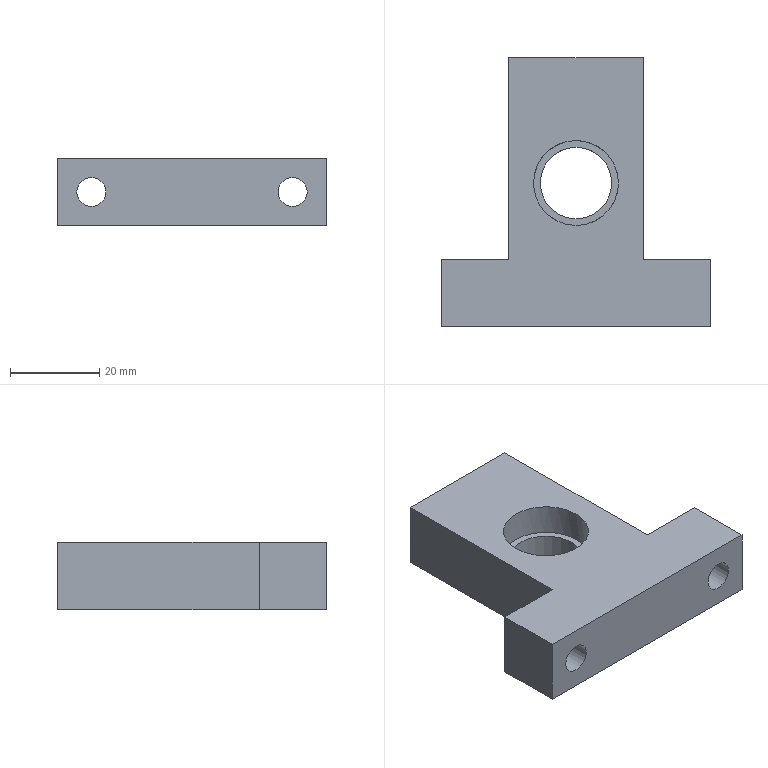Part | NX | features DATUM_CSYS 4, SKETCH 3, CBORE_HOLE 2, EXTRUDE 2, HOLE PACKAGE 1 | 1 solid | 19 faces | box 60 x 60 x 15 mm | volume 28357 mm3 | plane 13 | cylinder 6 | commonest cylinder face diameters 6.5 x2 11 x2 16 x1 19 x1
STEP:
#1=CARTESIAN_POINT('',(9.5,32.,15.));
#2=VERTEX_POINT('',#1);
#3=CARTESIAN_POINT('',(0.,32.,15.));
#4=DIRECTION('',(0.,0.,1.));
#5=DIRECTION('',(1.,0.,0.));
#6=AXIS2_PLACEMENT_3D('',#3,#4,#5);
#7=CIRCLE('',#6,9.5);
#8=EDGE_CURVE('',#2,#2,#7,.T.);
#9=ORIENTED_EDGE('',*,*,#8,.T.);
#10=EDGE_LOOP('',(#9));
#11=FACE_BOUND('',#10,.T.);
#12=CARTESIAN_POINT('',(0.,22.5,8.));
#13=VERTEX_POINT('',#12);
#14=CARTESIAN_POINT('',(0.,32.,8.));
#15=DIRECTION('',(0.,0.,-1.));
#16=DIRECTION('',(0.,-1.,0.));
#17=AXIS2_PLACEMENT_3D('',#14,#15,#16);
#18=CIRCLE('',#17,9.5);
#19=EDGE_CURVE('',#13,#13,#18,.T.);
#20=ORIENTED_EDGE('',*,*,#19,.T.);
#21=EDGE_LOOP('',(#20));
#22=FACE_BOUND('',#21,.T.);
#23=CARTESIAN_POINT('',(0.,32.,15.));
#24=DIRECTION('',(0.,0.,-1.));
#25=DIRECTION('',(-1.,0.,0.));
#26=AXIS2_PLACEMENT_3D('',#23,#24,#25);
#27=CYLINDRICAL_SURFACE('',#26,9.5);
#28=ADVANCED_FACE('',(#11,#22),#27,.F.);
#29=CARTESIAN_POINT('',(-30.,15.,0.));
#30=VERTEX_POINT('',#29);
#31=CARTESIAN_POINT('',(-30.,0.,0.));
#32=VERTEX_POINT('',#31);
#33=CARTESIAN_POINT('',(-30.,15.,0.));
#34=DIRECTION('',(0.,-1.,0.));
#35=VECTOR('',#34,1000.);
#36=LINE('',#33,#35);
#37=EDGE_CURVE('',#30,#32,#36,.T.);
#38=ORIENTED_EDGE('',*,*,#37,.T.);
#39=CARTESIAN_POINT('',(-30.,0.,15.));
#40=VERTEX_POINT('',#39);
#41=CARTESIAN_POINT('',(-30.,0.,15.));
#42=DIRECTION('',(0.,0.,-1.));
#43=VECTOR('',#42,1000.);
#44=LINE('',#41,#43);
#45=EDGE_CURVE('',#40,#32,#44,.T.);
#46=ORIENTED_EDGE('',*,*,#45,.F.);
#47=CARTESIAN_POINT('',(-30.,15.,15.));
#48=VERTEX_POINT('',#47);
#49=CARTESIAN_POINT('',(-30.,15.,15.));
#50=DIRECTION('',(0.,-1.,0.));
#51=VECTOR('',#50,1000.);
#52=LINE('',#49,#51);
#53=EDGE_CURVE('',#48,#40,#52,.T.);
#54=ORIENTED_EDGE('',*,*,#53,.F.);
#55=CARTESIAN_POINT('',(-30.,15.,15.));
#56=DIRECTION('',(0.,0.,-1.));
#57=VECTOR('',#56,1000.);
#58=LINE('',#55,#57);
#59=EDGE_CURVE('',#48,#30,#58,.T.);
#60=ORIENTED_EDGE('',*,*,#59,.T.);
#61=EDGE_LOOP('',(#38,#46,#54,#60));
#62=FACE_BOUND('',#61,.T.);
#63=CARTESIAN_POINT('',(-30.,15.,15.));
#64=DIRECTION('',(1.,0.,0.));
#65=DIRECTION('',(0.,0.,-1.));
#66=AXIS2_PLACEMENT_3D('',#63,#64,#65);
#67=PLANE('',#66);
#68=ADVANCED_FACE('',(#62),#67,.F.);
#69=CARTESIAN_POINT('',(19.25,0.,7.5));
#70=VERTEX_POINT('',#69);
#71=CARTESIAN_POINT('',(22.5,0.,7.5));
#72=DIRECTION('',(0.,1.,0.));
#73=DIRECTION('',(-1.,0.,0.));
#74=AXIS2_PLACEMENT_3D('',#71,#72,#73);
#75=CIRCLE('',#74,3.25);
#76=EDGE_CURVE('',#70,#70,#75,.T.);
#77=ORIENTED_EDGE('',*,*,#76,.T.);
#78=EDGE_LOOP('',(#77));
#79=FACE_BOUND('',#78,.T.);
#80=CARTESIAN_POINT('',(-25.75,0.,7.5));
#81=VERTEX_POINT('',#80);
#82=CARTESIAN_POINT('',(-22.5,0.,7.5));
#83=DIRECTION('',(0.,1.,0.));
#84=DIRECTION('',(-1.,0.,0.));
#85=AXIS2_PLACEMENT_3D('',#82,#83,#84);
#86=CIRCLE('',#85,3.25);
#87=EDGE_CURVE('',#81,#81,#86,.T.);
#88=ORIENTED_EDGE('',*,*,#87,.T.);
#89=EDGE_LOOP('',(#88));
#90=FACE_BOUND('',#89,.T.);
#91=CARTESIAN_POINT('',(30.,0.,0.));
#92=VERTEX_POINT('',#91);
#93=CARTESIAN_POINT('',(15.,0.,0.));
#94=DIRECTION('',(1.,0.,0.));
#95=VECTOR('',#94,1000.);
#96=LINE('',#93,#95);
#97=EDGE_CURVE('',#32,#92,#96,.T.);
#98=ORIENTED_EDGE('',*,*,#97,.T.);
#99=CARTESIAN_POINT('',(30.,0.,15.));
#100=VERTEX_POINT('',#99);
#101=CARTESIAN_POINT('',(30.,0.,15.));
#102=DIRECTION('',(0.,0.,-1.));
#103=VECTOR('',#102,1000.);
#104=LINE('',#101,#103);
#105=EDGE_CURVE('',#100,#92,#104,.T.);
#106=ORIENTED_EDGE('',*,*,#105,.F.);
#107=CARTESIAN_POINT('',(-30.,0.,15.));
#108=DIRECTION('',(1.,0.,0.));
#109=VECTOR('',#108,1000.);
#110=LINE('',#107,#109);
#111=EDGE_CURVE('',#40,#100,#110,.T.);
#112=ORIENTED_EDGE('',*,*,#111,.F.);
#113=ORIENTED_EDGE('',*,*,#45,.T.);
#114=EDGE_LOOP('',(#98,#106,#112,#113));
#115=FACE_BOUND('',#114,.T.);
#116=CARTESIAN_POINT('',(15.,0.,15.));
#117=DIRECTION('',(0.,1.,0.));
#118=DIRECTION('',(-1.,0.,0.));
#119=AXIS2_PLACEMENT_3D('',#116,#117,#118);
#120=PLANE('',#119);
#121=ADVANCED_FACE('',(#79,#90,#115),#120,.F.);
#122=CARTESIAN_POINT('',(30.,15.,0.));
#123=VERTEX_POINT('',#122);
#124=CARTESIAN_POINT('',(30.,0.,0.));
#125=DIRECTION('',(0.,1.,0.));
#126=VECTOR('',#125,1000.);
#127=LINE('',#124,#126);
#128=EDGE_CURVE('',#92,#123,#127,.T.);
#129=ORIENTED_EDGE('',*,*,#128,.T.);
#130=CARTESIAN_POINT('',(30.,15.,15.));
#131=VERTEX_POINT('',#130);
#132=CARTESIAN_POINT('',(30.,15.,15.));
#133=DIRECTION('',(0.,0.,-1.));
#134=VECTOR('',#133,1000.);
#135=LINE('',#132,#134);
#136=EDGE_CURVE('',#131,#123,#135,.T.);
#137=ORIENTED_EDGE('',*,*,#136,.F.);
#138=CARTESIAN_POINT('',(30.,0.,15.));
#139=DIRECTION('',(0.,1.,0.));
#140=VECTOR('',#139,1000.);
#141=LINE('',#138,#140);
#142=EDGE_CURVE('',#100,#131,#141,.T.);
#143=ORIENTED_EDGE('',*,*,#142,.F.);
#144=ORIENTED_EDGE('',*,*,#105,.T.);
#145=EDGE_LOOP('',(#129,#137,#143,#144));
#146=FACE_BOUND('',#145,.T.);
#147=CARTESIAN_POINT('',(30.,0.,15.));
#148=DIRECTION('',(-1.,0.,0.));
#149=DIRECTION('',(0.,0.,1.));
#150=AXIS2_PLACEMENT_3D('',#147,#148,#149);
#151=PLANE('',#150);
#152=ADVANCED_FACE('',(#146),#151,.F.);
#153=CARTESIAN_POINT('',(28.,15.,7.5));
#154=VERTEX_POINT('',#153);
#155=CARTESIAN_POINT('',(22.5,15.,7.5));
#156=DIRECTION('',(0.,-1.,0.));
#157=DIRECTION('',(1.,0.,0.));
#158=AXIS2_PLACEMENT_3D('',#155,#156,#157);
#159=CIRCLE('',#158,5.5);
#160=EDGE_CURVE('',#154,#154,#159,.T.);
#161=ORIENTED_EDGE('',*,*,#160,.T.);
#162=EDGE_LOOP('',(#161));
#163=FACE_BOUND('',#162,.T.);
#164=CARTESIAN_POINT('',(15.,15.,0.));
#165=VERTEX_POINT('',#164);
#166=CARTESIAN_POINT('',(30.,15.,0.));
#167=DIRECTION('',(-1.,0.,0.));
#168=VECTOR('',#167,1000.);
#169=LINE('',#166,#168);
#170=EDGE_CURVE('',#123,#165,#169,.T.);
#171=ORIENTED_EDGE('',*,*,#170,.T.);
#172=CARTESIAN_POINT('',(15.,15.,15.));
#173=VERTEX_POINT('',#172);
#174=CARTESIAN_POINT('',(15.,15.,15.));
#175=DIRECTION('',(0.,0.,-1.));
#176=VECTOR('',#175,1000.);
#177=LINE('',#174,#176);
#178=EDGE_CURVE('',#173,#165,#177,.T.);
#179=ORIENTED_EDGE('',*,*,#178,.F.);
#180=CARTESIAN_POINT('',(30.,15.,15.));
#181=DIRECTION('',(-1.,0.,0.));
#182=VECTOR('',#181,1000.);
#183=LINE('',#180,#182);
#184=EDGE_CURVE('',#131,#173,#183,.T.);
#185=ORIENTED_EDGE('',*,*,#184,.F.);
#186=ORIENTED_EDGE('',*,*,#136,.T.);
#187=EDGE_LOOP('',(#171,#179,#185,#186));
#188=FACE_BOUND('',#187,.T.);
#189=CARTESIAN_POINT('',(30.,15.,15.));
#190=DIRECTION('',(0.,-1.,0.));
#191=DIRECTION('',(1.,0.,0.));
#192=AXIS2_PLACEMENT_3D('',#189,#190,#191);
#193=PLANE('',#192);
#194=ADVANCED_FACE('',(#163,#188),#193,.F.);
#195=CARTESIAN_POINT('',(15.,60.,0.));
#196=VERTEX_POINT('',#195);
#197=CARTESIAN_POINT('',(15.,15.,0.));
#198=DIRECTION('',(0.,1.,0.));
#199=VECTOR('',#198,1000.);
#200=LINE('',#197,#199);
#201=EDGE_CURVE('',#165,#196,#200,.T.);
#202=ORIENTED_EDGE('',*,*,#201,.T.);
#203=CARTESIAN_POINT('',(15.,60.,15.));
#204=VERTEX_POINT('',#203);
#205=CARTESIAN_POINT('',(15.,60.,15.));
#206=DIRECTION('',(0.,0.,-1.));
#207=VECTOR('',#206,1000.);
#208=LINE('',#205,#207);
#209=EDGE_CURVE('',#204,#196,#208,.T.);
#210=ORIENTED_EDGE('',*,*,#209,.F.);
#211=CARTESIAN_POINT('',(15.,15.,15.));
#212=DIRECTION('',(0.,1.,0.));
#213=VECTOR('',#212,1000.);
#214=LINE('',#211,#213);
#215=EDGE_CURVE('',#173,#204,#214,.T.);
#216=ORIENTED_EDGE('',*,*,#215,.F.);
#217=ORIENTED_EDGE('',*,*,#178,.T.);
#218=EDGE_LOOP('',(#202,#210,#216,#217));
#219=FACE_BOUND('',#218,.T.);
#220=CARTESIAN_POINT('',(15.,15.,15.));
#221=DIRECTION('',(-1.,0.,0.));
#222=DIRECTION('',(0.,-1.,0.));
#223=AXIS2_PLACEMENT_3D('',#220,#221,#222);
#224=PLANE('',#223);
#225=ADVANCED_FACE('',(#219),#224,.F.);
#226=CARTESIAN_POINT('',(-15.,60.,0.));
#227=VERTEX_POINT('',#226);
#228=CARTESIAN_POINT('',(15.,60.,0.));
#229=DIRECTION('',(-1.,0.,0.));
#230=VECTOR('',#229,1000.);
#231=LINE('',#228,#230);
#232=EDGE_CURVE('',#196,#227,#231,.T.);
#233=ORIENTED_EDGE('',*,*,#232,.T.);
#234=CARTESIAN_POINT('',(-15.,60.,15.));
#235=VERTEX_POINT('',#234);
#236=CARTESIAN_POINT('',(-15.,60.,15.));
#237=DIRECTION('',(0.,0.,-1.));
#238=VECTOR('',#237,1000.);
#239=LINE('',#236,#238);
#240=EDGE_CURVE('',#235,#227,#239,.T.);
#241=ORIENTED_EDGE('',*,*,#240,.F.);
#242=CARTESIAN_POINT('',(15.,60.,15.));
#243=DIRECTION('',(-1.,0.,0.));
#244=VECTOR('',#243,1000.);
#245=LINE('',#242,#244);
#246=EDGE_CURVE('',#204,#235,#245,.T.);
#247=ORIENTED_EDGE('',*,*,#246,.F.);
#248=ORIENTED_EDGE('',*,*,#209,.T.);
#249=EDGE_LOOP('',(#233,#241,#247,#248));
#250=FACE_BOUND('',#249,.T.);
#251=CARTESIAN_POINT('',(15.,60.,15.));
#252=DIRECTION('',(0.,-1.,0.));
#253=DIRECTION('',(0.,0.,-1.));
#254=AXIS2_PLACEMENT_3D('',#251,#252,#253);
#255=PLANE('',#254);
#256=ADVANCED_FACE('',(#250),#255,.F.);
#257=CARTESIAN_POINT('',(-15.,15.,0.));
#258=VERTEX_POINT('',#257);
#259=CARTESIAN_POINT('',(-15.,60.,0.));
#260=DIRECTION('',(0.,-1.,0.));
#261=VECTOR('',#260,1000.);
#262=LINE('',#259,#261);
#263=EDGE_CURVE('',#227,#258,#262,.T.);
#264=ORIENTED_EDGE('',*,*,#263,.T.);
#265=CARTESIAN_POINT('',(-15.,15.,15.));
#266=VERTEX_POINT('',#265);
#267=CARTESIAN_POINT('',(-15.,15.,15.));
#268=DIRECTION('',(0.,0.,-1.));
#269=VECTOR('',#268,1000.);
#270=LINE('',#267,#269);
#271=EDGE_CURVE('',#266,#258,#270,.T.);
#272=ORIENTED_EDGE('',*,*,#271,.F.);
#273=CARTESIAN_POINT('',(-15.,60.,15.));
#274=DIRECTION('',(0.,-1.,0.));
#275=VECTOR('',#274,1000.);
#276=LINE('',#273,#275);
#277=EDGE_CURVE('',#235,#266,#276,.T.);
#278=ORIENTED_EDGE('',*,*,#277,.F.);
#279=ORIENTED_EDGE('',*,*,#240,.T.);
#280=EDGE_LOOP('',(#264,#272,#278,#279));
#281=FACE_BOUND('',#280,.T.);
#282=CARTESIAN_POINT('',(-15.,60.,15.));
#283=DIRECTION('',(1.,0.,0.));
#284=DIRECTION('',(0.,1.,0.));
#285=AXIS2_PLACEMENT_3D('',#282,#283,#284);
#286=PLANE('',#285);
#287=ADVANCED_FACE('',(#281),#286,.F.);
#288=CARTESIAN_POINT('',(-17.,15.,7.5));
#289=VERTEX_POINT('',#288);
#290=CARTESIAN_POINT('',(-22.5,15.,7.5));
#291=DIRECTION('',(0.,-1.,0.));
#292=DIRECTION('',(1.,0.,0.));
#293=AXIS2_PLACEMENT_3D('',#290,#291,#292);
#294=CIRCLE('',#293,5.5);
#295=EDGE_CURVE('',#289,#289,#294,.T.);
#296=ORIENTED_EDGE('',*,*,#295,.T.);
#297=EDGE_LOOP('',(#296));
#298=FACE_BOUND('',#297,.T.);
#299=CARTESIAN_POINT('',(-15.,15.,0.));
#300=DIRECTION('',(-1.,0.,0.));
#301=VECTOR('',#300,1000.);
#302=LINE('',#299,#301);
#303=EDGE_CURVE('',#258,#30,#302,.T.);
#304=ORIENTED_EDGE('',*,*,#303,.T.);
#305=ORIENTED_EDGE('',*,*,#59,.F.);
#306=CARTESIAN_POINT('',(-15.,15.,15.));
#307=DIRECTION('',(-1.,0.,0.));
#308=VECTOR('',#307,1000.);
#309=LINE('',#306,#308);
#310=EDGE_CURVE('',#266,#48,#309,.T.);
#311=ORIENTED_EDGE('',*,*,#310,.F.);
#312=ORIENTED_EDGE('',*,*,#271,.T.);
#313=EDGE_LOOP('',(#304,#305,#311,#312));
#314=FACE_BOUND('',#313,.T.);
#315=CARTESIAN_POINT('',(-15.,15.,15.));
#316=DIRECTION('',(0.,-1.,0.));
#317=DIRECTION('',(1.,0.,0.));
#318=AXIS2_PLACEMENT_3D('',#315,#316,#317);
#319=PLANE('',#318);
#320=ADVANCED_FACE('',(#298,#314),#319,.F.);
#321=ORIENTED_EDGE('',*,*,#53,.T.);
#322=ORIENTED_EDGE('',*,*,#111,.T.);
#323=ORIENTED_EDGE('',*,*,#142,.T.);
#324=ORIENTED_EDGE('',*,*,#184,.T.);
#325=ORIENTED_EDGE('',*,*,#215,.T.);
#326=ORIENTED_EDGE('',*,*,#246,.T.);
#327=ORIENTED_EDGE('',*,*,#277,.T.);
#328=ORIENTED_EDGE('',*,*,#310,.T.);
#329=EDGE_LOOP('',(#321,#322,#323,#324,#325,#326,#327,#328));
#330=FACE_BOUND('',#329,.T.);
#331=ORIENTED_EDGE('',*,*,#8,.F.);
#332=EDGE_LOOP('',(#331));
#333=FACE_BOUND('',#332,.T.);
#334=CARTESIAN_POINT('',(0.,32.,15.));
#335=DIRECTION('',(0.,0.,1.));
#336=DIRECTION('',(1.,0.,0.));
#337=AXIS2_PLACEMENT_3D('',#334,#335,#336);
#338=PLANE('',#337);
#339=ADVANCED_FACE('',(#330,#333),#338,.T.);
#340=ORIENTED_EDGE('',*,*,#37,.F.);
#341=ORIENTED_EDGE('',*,*,#303,.F.);
#342=ORIENTED_EDGE('',*,*,#263,.F.);
#343=ORIENTED_EDGE('',*,*,#232,.F.);
#344=ORIENTED_EDGE('',*,*,#201,.F.);
#345=ORIENTED_EDGE('',*,*,#170,.F.);
#346=ORIENTED_EDGE('',*,*,#128,.F.);
#347=ORIENTED_EDGE('',*,*,#97,.F.);
#348=EDGE_LOOP('',(#340,#341,#342,#343,#344,#345,#346,#347));
#349=FACE_BOUND('',#348,.T.);
#350=CARTESIAN_POINT('',(0.,24.,0.));
#351=VERTEX_POINT('',#350);
#352=CARTESIAN_POINT('',(0.,32.,0.));
#353=DIRECTION('',(0.,0.,-1.));
#354=DIRECTION('',(0.,-1.,0.));
#355=AXIS2_PLACEMENT_3D('',#352,#353,#354);
#356=CIRCLE('',#355,8.);
#357=EDGE_CURVE('',#351,#351,#356,.T.);
#358=ORIENTED_EDGE('',*,*,#357,.F.);
#359=EDGE_LOOP('',(#358));
#360=FACE_BOUND('',#359,.T.);
#361=CARTESIAN_POINT('',(0.,32.,0.));
#362=DIRECTION('',(0.,0.,1.));
#363=DIRECTION('',(1.,0.,0.));
#364=AXIS2_PLACEMENT_3D('',#361,#362,#363);
#365=PLANE('',#364);
#366=ADVANCED_FACE('',(#349,#360),#365,.F.);
#367=CARTESIAN_POINT('',(0.,24.,8.));
#368=VERTEX_POINT('',#367);
#369=CARTESIAN_POINT('',(0.,32.,8.));
#370=DIRECTION('',(0.,0.,-1.));
#371=DIRECTION('',(0.,-1.,0.));
#372=AXIS2_PLACEMENT_3D('',#369,#370,#371);
#373=CIRCLE('',#372,8.);
#374=EDGE_CURVE('',#368,#368,#373,.T.);
#375=ORIENTED_EDGE('',*,*,#374,.F.);
#376=EDGE_LOOP('',(#375));
#377=FACE_BOUND('',#376,.T.);
#378=ORIENTED_EDGE('',*,*,#357,.T.);
#379=EDGE_LOOP('',(#378));
#380=FACE_BOUND('',#379,.T.);
#381=CARTESIAN_POINT('',(0.,32.,8.));
#382=DIRECTION('',(0.,0.,-1.));
#383=DIRECTION('',(-1.,0.,0.));
#384=AXIS2_PLACEMENT_3D('',#381,#382,#383);
#385=CYLINDRICAL_SURFACE('',#384,8.);
#386=ADVANCED_FACE('',(#377,#380),#385,.F.);
#387=ORIENTED_EDGE('',*,*,#19,.F.);
#388=EDGE_LOOP('',(#387));
#389=FACE_BOUND('',#388,.T.);
#390=ORIENTED_EDGE('',*,*,#374,.T.);
#391=EDGE_LOOP('',(#390));
#392=FACE_BOUND('',#391,.T.);
#393=CARTESIAN_POINT('',(0.,32.,8.));
#394=DIRECTION('',(0.,0.,-1.));
#395=DIRECTION('',(-1.,0.,0.));
#396=AXIS2_PLACEMENT_3D('',#393,#394,#395);
#397=PLANE('',#396);
#398=ADVANCED_FACE('',(#389,#392),#397,.F.);
#399=CARTESIAN_POINT('',(-19.25,8.5,7.5));
#400=VERTEX_POINT('',#399);
#401=CARTESIAN_POINT('',(-22.5,8.5,7.5));
#402=DIRECTION('',(0.,-1.,0.));
#403=DIRECTION('',(1.,0.,0.));
#404=AXIS2_PLACEMENT_3D('',#401,#402,#403);
#405=CIRCLE('',#404,3.25);
#406=EDGE_CURVE('',#400,#400,#405,.F.);
#407=ORIENTED_EDGE('',*,*,#406,.T.);
#408=EDGE_LOOP('',(#407));
#409=FACE_BOUND('',#408,.T.);
#410=ORIENTED_EDGE('',*,*,#87,.F.);
#411=EDGE_LOOP('',(#410));
#412=FACE_BOUND('',#411,.T.);
#413=CARTESIAN_POINT('',(-22.5,-11.711,7.5));
#414=DIRECTION('',(0.,-1.,0.));
#415=DIRECTION('',(1.,0.,0.));
#416=AXIS2_PLACEMENT_3D('',#413,#414,#415);
#417=CYLINDRICAL_SURFACE('',#416,3.25);
#418=ADVANCED_FACE('',(#409,#412),#417,.F.);
#419=ORIENTED_EDGE('',*,*,#406,.F.);
#420=EDGE_LOOP('',(#419));
#421=FACE_BOUND('',#420,.T.);
#422=CARTESIAN_POINT('',(-17.,8.5,7.5));
#423=VERTEX_POINT('',#422);
#424=CARTESIAN_POINT('',(-22.5,8.5,7.5));
#425=DIRECTION('',(0.,-1.,0.));
#426=DIRECTION('',(1.,0.,0.));
#427=AXIS2_PLACEMENT_3D('',#424,#425,#426);
#428=CIRCLE('',#427,5.5);
#429=EDGE_CURVE('',#423,#423,#428,.F.);
#430=ORIENTED_EDGE('',*,*,#429,.T.);
#431=EDGE_LOOP('',(#430));
#432=FACE_BOUND('',#431,.T.);
#433=CARTESIAN_POINT('',(-22.5,8.5,7.5));
#434=DIRECTION('',(0.,-1.,0.));
#435=DIRECTION('',(1.,0.,0.));
#436=AXIS2_PLACEMENT_3D('',#433,#434,#435);
#437=PLANE('',#436);
#438=ADVANCED_FACE('',(#421,#432),#437,.F.);
#439=ORIENTED_EDGE('',*,*,#429,.F.);
#440=EDGE_LOOP('',(#439));
#441=FACE_BOUND('',#440,.T.);
#442=ORIENTED_EDGE('',*,*,#295,.F.);
#443=EDGE_LOOP('',(#442));
#444=FACE_BOUND('',#443,.T.);
#445=CARTESIAN_POINT('',(-22.5,15.,7.5));
#446=DIRECTION('',(0.,-1.,0.));
#447=DIRECTION('',(1.,0.,0.));
#448=AXIS2_PLACEMENT_3D('',#445,#446,#447);
#449=CYLINDRICAL_SURFACE('',#448,5.5);
#450=ADVANCED_FACE('',(#441,#444),#449,.F.);
#451=CARTESIAN_POINT('',(25.75,8.5,7.5));
#452=VERTEX_POINT('',#451);
#453=CARTESIAN_POINT('',(22.5,8.5,7.5));
#454=DIRECTION('',(0.,-1.,0.));
#455=DIRECTION('',(1.,0.,0.));
#456=AXIS2_PLACEMENT_3D('',#453,#454,#455);
#457=CIRCLE('',#456,3.25);
#458=EDGE_CURVE('',#452,#452,#457,.F.);
#459=ORIENTED_EDGE('',*,*,#458,.T.);
#460=EDGE_LOOP('',(#459));
#461=FACE_BOUND('',#460,.T.);
#462=ORIENTED_EDGE('',*,*,#76,.F.);
#463=EDGE_LOOP('',(#462));
#464=FACE_BOUND('',#463,.T.);
#465=CARTESIAN_POINT('',(22.5,-11.711,7.5));
#466=DIRECTION('',(0.,-1.,0.));
#467=DIRECTION('',(1.,0.,0.));
#468=AXIS2_PLACEMENT_3D('',#465,#466,#467);
#469=CYLINDRICAL_SURFACE('',#468,3.25);
#470=ADVANCED_FACE('',(#461,#464),#469,.F.);
#471=ORIENTED_EDGE('',*,*,#458,.F.);
#472=EDGE_LOOP('',(#471));
#473=FACE_BOUND('',#472,.T.);
#474=CARTESIAN_POINT('',(28.,8.5,7.5));
#475=VERTEX_POINT('',#474);
#476=CARTESIAN_POINT('',(22.5,8.5,7.5));
#477=DIRECTION('',(0.,-1.,0.));
#478=DIRECTION('',(1.,0.,0.));
#479=AXIS2_PLACEMENT_3D('',#476,#477,#478);
#480=CIRCLE('',#479,5.5);
#481=EDGE_CURVE('',#475,#475,#480,.F.);
#482=ORIENTED_EDGE('',*,*,#481,.T.);
#483=EDGE_LOOP('',(#482));
#484=FACE_BOUND('',#483,.T.);
#485=CARTESIAN_POINT('',(22.5,8.5,7.5));
#486=DIRECTION('',(0.,-1.,0.));
#487=DIRECTION('',(1.,0.,0.));
#488=AXIS2_PLACEMENT_3D('',#485,#486,#487);
#489=PLANE('',#488);
#490=ADVANCED_FACE('',(#473,#484),#489,.F.);
#491=ORIENTED_EDGE('',*,*,#481,.F.);
#492=EDGE_LOOP('',(#491));
#493=FACE_BOUND('',#492,.T.);
#494=ORIENTED_EDGE('',*,*,#160,.F.);
#495=EDGE_LOOP('',(#494));
#496=FACE_BOUND('',#495,.T.);
#497=CARTESIAN_POINT('',(22.5,15.,7.5));
#498=DIRECTION('',(0.,-1.,0.));
#499=DIRECTION('',(1.,0.,0.));
#500=AXIS2_PLACEMENT_3D('',#497,#498,#499);
#501=CYLINDRICAL_SURFACE('',#500,5.5);
#502=ADVANCED_FACE('',(#493,#496),#501,.F.);
#503=CLOSED_SHELL('',(#28,#68,#121,#152,#194,#225,#256,#287,#320,#339,#366,#386,#398,#418,#438,#450,#470,#490,#502));
#504=MANIFOLD_SOLID_BREP('',#503);
#505=(LENGTH_UNIT()NAMED_UNIT(*)SI_UNIT(.MILLI.,.METRE.));
#506=UNCERTAINTY_MEASURE_WITH_UNIT(LENGTH_MEASURE(0.00001),#505,'','');
#507=(NAMED_UNIT(*)PLANE_ANGLE_UNIT()SI_UNIT($,.RADIAN.));
#508=(NAMED_UNIT(*)SI_UNIT($,.STERADIAN.)SOLID_ANGLE_UNIT());
#509=(GEOMETRIC_REPRESENTATION_CONTEXT(3)GLOBAL_UNCERTAINTY_ASSIGNED_CONTEXT((#506))GLOBAL_UNIT_ASSIGNED_CONTEXT((#505,#507,#508))REPRESENTATION_CONTEXT('',''));
#510=ADVANCED_BREP_SHAPE_REPRESENTATION('',(#504),#509);